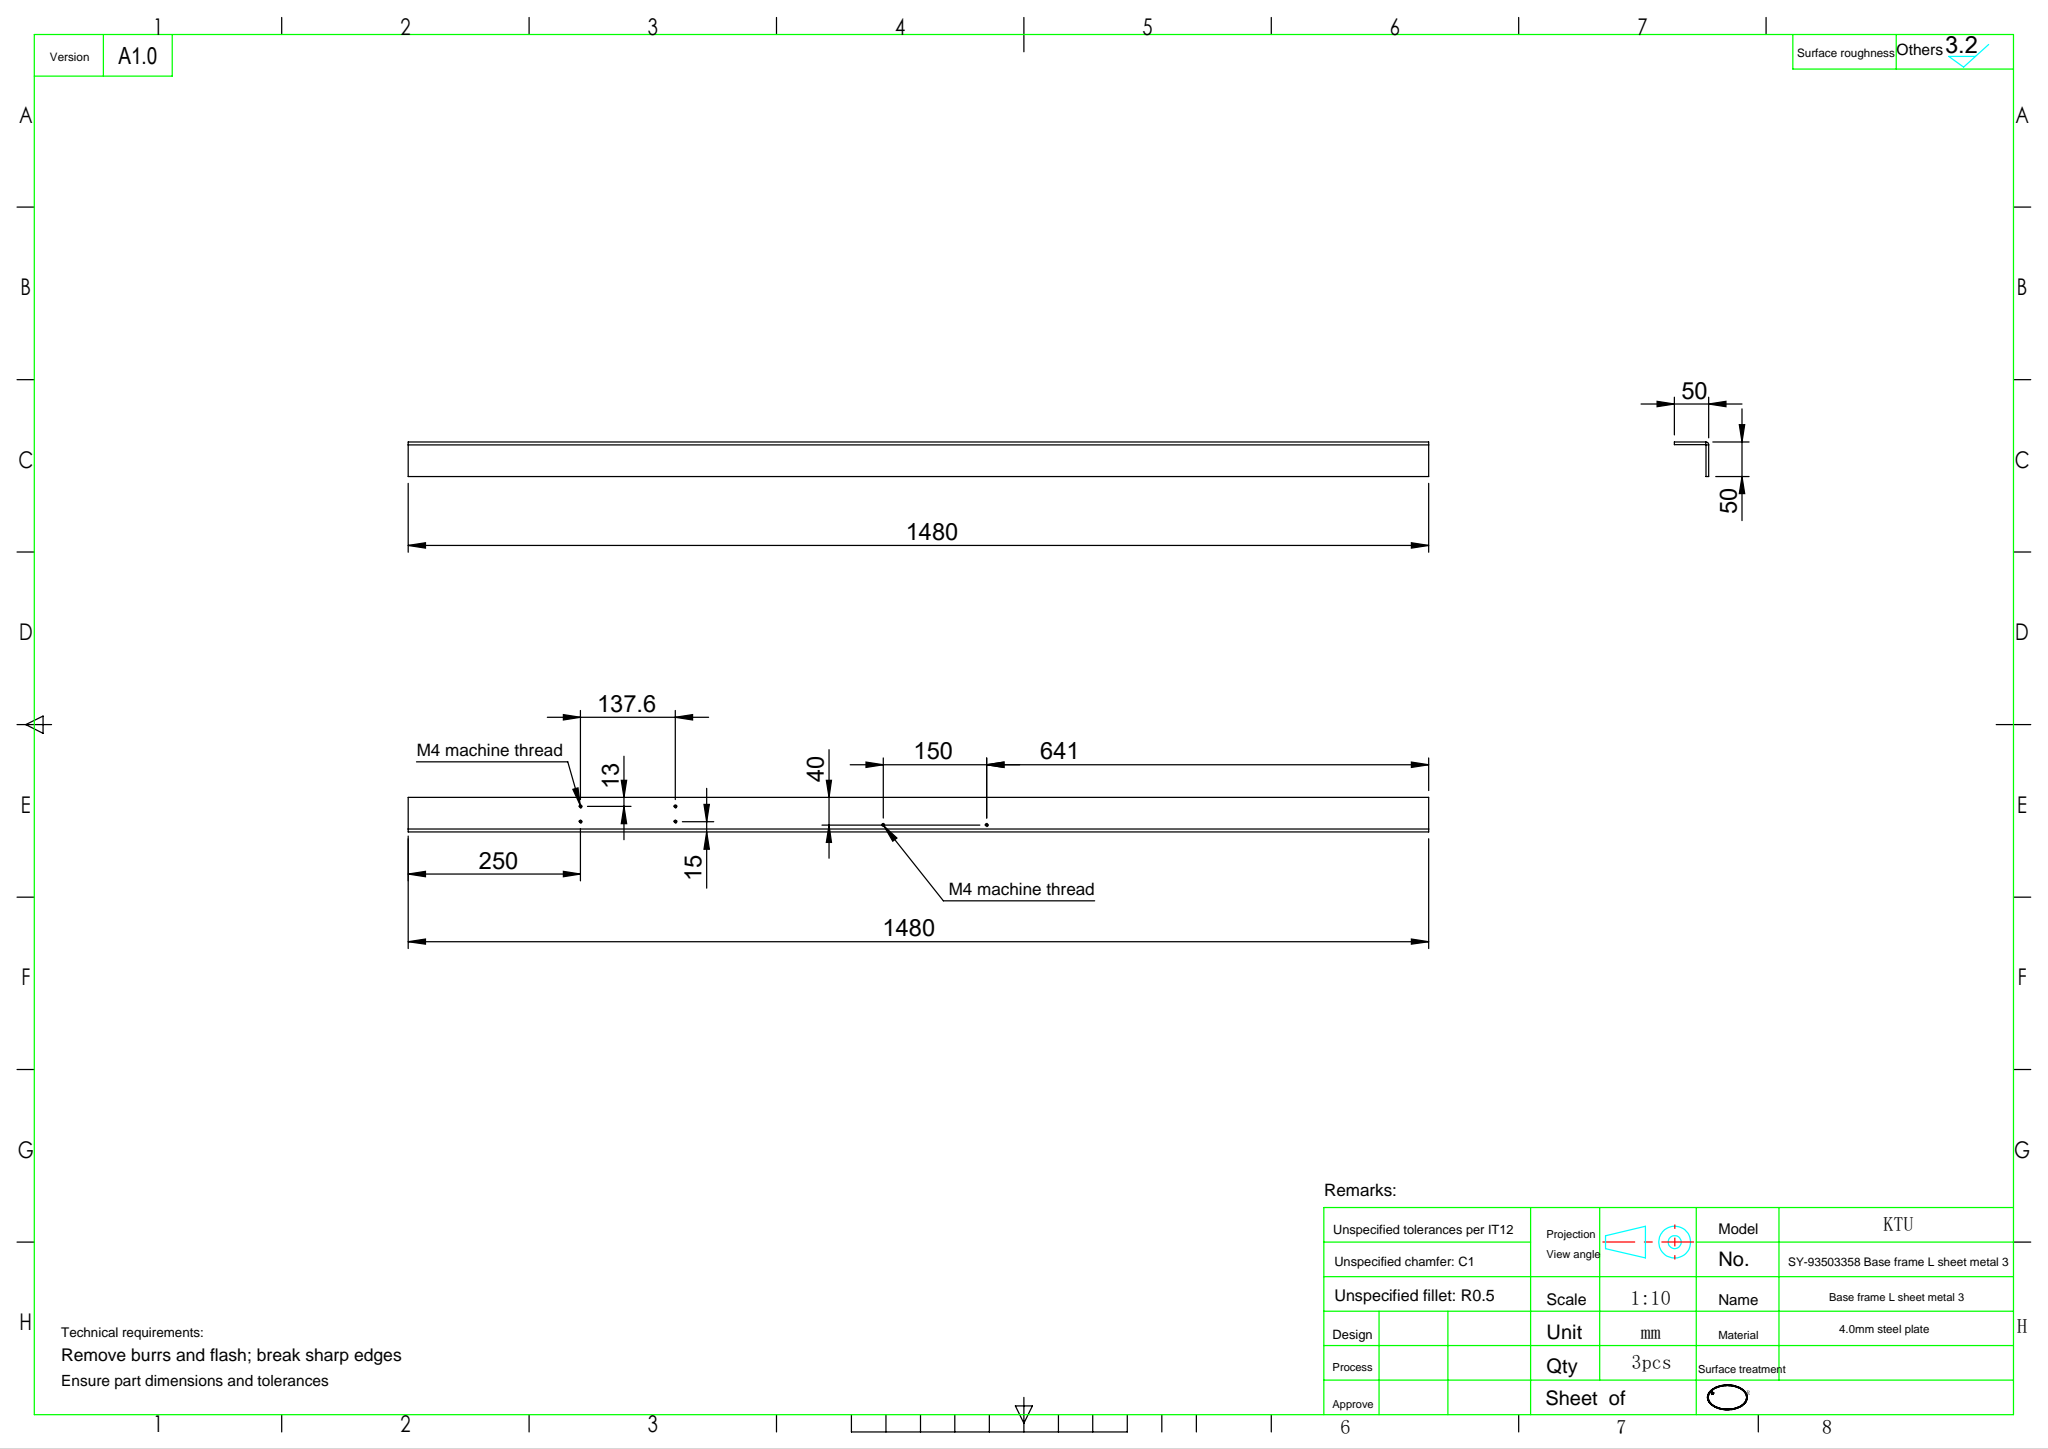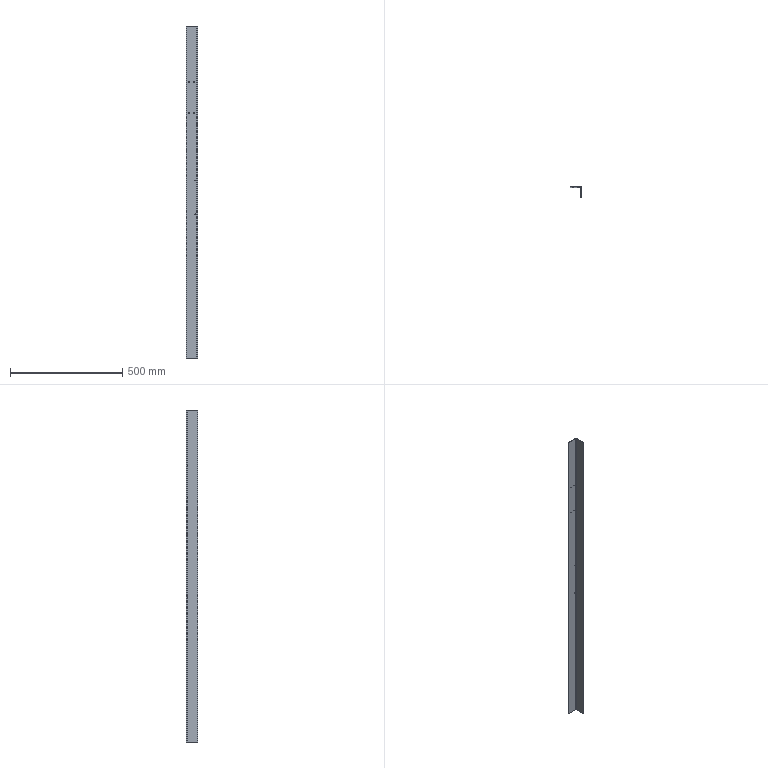Part | SolidWorks | features Cut 2, FlatPattern 1, SMBaseFlange 1, SheetMetal 1 | 1 solid | 26 faces | box 50 x 50 x 1480 mm | volume 562525 mm3 | cylinder 14 | plane 12 | commonest cylinder face diameters 3.3 x8 3.299 x4 0.4 x1 8.4 x1
STEP:
#1=CARTESIAN_POINT('',(-15.,-4.,1228.351));
#2=VERTEX_POINT('',#1);
#3=CARTESIAN_POINT('',(-15.,-4.,1231.649));
#4=VERTEX_POINT('',#3);
#5=CARTESIAN_POINT('',(-15.,-4.,1230.));
#6=DIRECTION('',(0.,1.,0.));
#7=DIRECTION('',(0.,0.,1.));
#8=AXIS2_PLACEMENT_3D('',#5,#6,#7);
#9=CIRCLE('',#8,1.649);
#10=EDGE_CURVE('',#2,#4,#9,.T.);
#11=ORIENTED_EDGE('',*,*,#10,.F.);
#12=CARTESIAN_POINT('',(-15.,0.,1228.351));
#13=VERTEX_POINT('',#12);
#14=CARTESIAN_POINT('',(-15.,-10.,1228.351));
#15=DIRECTION('',(0.,1.,0.));
#16=VECTOR('',#15,1000.);
#17=LINE('',#14,#16);
#18=EDGE_CURVE('',#2,#13,#17,.T.);
#19=ORIENTED_EDGE('',*,*,#18,.T.);
#20=CARTESIAN_POINT('',(-15.,0.,1231.649));
#21=VERTEX_POINT('',#20);
#22=CARTESIAN_POINT('',(-15.,0.,1230.));
#23=DIRECTION('',(0.,1.,0.));
#24=DIRECTION('',(0.,0.,1.));
#25=AXIS2_PLACEMENT_3D('',#22,#23,#24);
#26=CIRCLE('',#25,1.649);
#27=EDGE_CURVE('',#13,#21,#26,.T.);
#28=ORIENTED_EDGE('',*,*,#27,.T.);
#29=CARTESIAN_POINT('',(-15.,-10.,1231.649));
#30=DIRECTION('',(0.,1.,0.));
#31=VECTOR('',#30,1000.);
#32=LINE('',#29,#31);
#33=EDGE_CURVE('',#4,#21,#32,.T.);
#34=ORIENTED_EDGE('',*,*,#33,.F.);
#35=EDGE_LOOP('',(#11,#19,#28,#34));
#36=FACE_OUTER_BOUND('',#35,.T.);
#37=CARTESIAN_POINT('',(-15.,-10.,1230.));
#38=DIRECTION('',(0.,1.,0.));
#39=DIRECTION('',(0.,0.,1.));
#40=AXIS2_PLACEMENT_3D('',#37,#38,#39);
#41=CYLINDRICAL_SURFACE('',#40,1.649);
#42=ADVANCED_FACE('',(#36),#41,.F.);
#43=CARTESIAN_POINT('',(-15.,-4.,1090.751));
#44=VERTEX_POINT('',#43);
#45=CARTESIAN_POINT('',(-15.,-4.,1094.049));
#46=VERTEX_POINT('',#45);
#47=CARTESIAN_POINT('',(-15.,-4.,1092.4));
#48=DIRECTION('',(0.,1.,0.));
#49=DIRECTION('',(0.,0.,1.));
#50=AXIS2_PLACEMENT_3D('',#47,#48,#49);
#51=CIRCLE('',#50,1.649);
#52=EDGE_CURVE('',#44,#46,#51,.T.);
#53=ORIENTED_EDGE('',*,*,#52,.F.);
#54=CARTESIAN_POINT('',(-15.,0.,1090.751));
#55=VERTEX_POINT('',#54);
#56=CARTESIAN_POINT('',(-15.,-10.,1090.751));
#57=DIRECTION('',(0.,1.,0.));
#58=VECTOR('',#57,1000.);
#59=LINE('',#56,#58);
#60=EDGE_CURVE('',#44,#55,#59,.T.);
#61=ORIENTED_EDGE('',*,*,#60,.T.);
#62=CARTESIAN_POINT('',(-15.,0.,1094.049));
#63=VERTEX_POINT('',#62);
#64=CARTESIAN_POINT('',(-15.,0.,1092.4));
#65=DIRECTION('',(0.,1.,0.));
#66=DIRECTION('',(0.,0.,1.));
#67=AXIS2_PLACEMENT_3D('',#64,#65,#66);
#68=CIRCLE('',#67,1.649);
#69=EDGE_CURVE('',#55,#63,#68,.T.);
#70=ORIENTED_EDGE('',*,*,#69,.T.);
#71=CARTESIAN_POINT('',(-15.,-10.,1094.049));
#72=DIRECTION('',(0.,1.,0.));
#73=VECTOR('',#72,1000.);
#74=LINE('',#71,#73);
#75=EDGE_CURVE('',#46,#63,#74,.T.);
#76=ORIENTED_EDGE('',*,*,#75,.F.);
#77=EDGE_LOOP('',(#53,#61,#70,#76));
#78=FACE_OUTER_BOUND('',#77,.T.);
#79=CARTESIAN_POINT('',(-15.,-10.,1092.4));
#80=DIRECTION('',(0.,1.,0.));
#81=DIRECTION('',(0.,0.,1.));
#82=AXIS2_PLACEMENT_3D('',#79,#80,#81);
#83=CYLINDRICAL_SURFACE('',#82,1.649);
#84=ADVANCED_FACE('',(#78),#83,.F.);
#85=CARTESIAN_POINT('',(-10.,-4.,639.35));
#86=VERTEX_POINT('',#85);
#87=CARTESIAN_POINT('',(-10.,-4.,642.65));
#88=VERTEX_POINT('',#87);
#89=CARTESIAN_POINT('',(-10.,-4.,641.));
#90=DIRECTION('',(0.,1.,0.));
#91=DIRECTION('',(0.,0.,1.));
#92=AXIS2_PLACEMENT_3D('',#89,#90,#91);
#93=CIRCLE('',#92,1.65);
#94=EDGE_CURVE('',#86,#88,#93,.T.);
#95=ORIENTED_EDGE('',*,*,#94,.F.);
#96=CARTESIAN_POINT('',(-10.,0.,639.35));
#97=VERTEX_POINT('',#96);
#98=CARTESIAN_POINT('',(-10.,-10.,639.35));
#99=DIRECTION('',(0.,1.,0.));
#100=VECTOR('',#99,1000.);
#101=LINE('',#98,#100);
#102=EDGE_CURVE('',#86,#97,#101,.T.);
#103=ORIENTED_EDGE('',*,*,#102,.T.);
#104=CARTESIAN_POINT('',(-10.,0.,642.65));
#105=VERTEX_POINT('',#104);
#106=CARTESIAN_POINT('',(-10.,0.,641.));
#107=DIRECTION('',(0.,1.,0.));
#108=DIRECTION('',(0.,0.,1.));
#109=AXIS2_PLACEMENT_3D('',#106,#107,#108);
#110=CIRCLE('',#109,1.65);
#111=EDGE_CURVE('',#97,#105,#110,.T.);
#112=ORIENTED_EDGE('',*,*,#111,.T.);
#113=CARTESIAN_POINT('',(-10.,-10.,642.65));
#114=DIRECTION('',(0.,1.,0.));
#115=VECTOR('',#114,1000.);
#116=LINE('',#113,#115);
#117=EDGE_CURVE('',#88,#105,#116,.T.);
#118=ORIENTED_EDGE('',*,*,#117,.F.);
#119=EDGE_LOOP('',(#95,#103,#112,#118));
#120=FACE_OUTER_BOUND('',#119,.T.);
#121=CARTESIAN_POINT('',(-10.,-10.,641.));
#122=DIRECTION('',(0.,1.,0.));
#123=DIRECTION('',(0.,0.,1.));
#124=AXIS2_PLACEMENT_3D('',#121,#122,#123);
#125=CYLINDRICAL_SURFACE('',#124,1.65);
#126=ADVANCED_FACE('',(#120),#125,.F.);
#127=CARTESIAN_POINT('',(-37.,-4.,1228.35));
#128=VERTEX_POINT('',#127);
#129=CARTESIAN_POINT('',(-37.,-4.,1231.65));
#130=VERTEX_POINT('',#129);
#131=CARTESIAN_POINT('',(-37.,-4.,1230.));
#132=DIRECTION('',(0.,1.,0.));
#133=DIRECTION('',(0.,0.,1.));
#134=AXIS2_PLACEMENT_3D('',#131,#132,#133);
#135=CIRCLE('',#134,1.65);
#136=EDGE_CURVE('',#128,#130,#135,.T.);
#137=ORIENTED_EDGE('',*,*,#136,.F.);
#138=CARTESIAN_POINT('',(-37.,0.,1228.35));
#139=VERTEX_POINT('',#138);
#140=CARTESIAN_POINT('',(-37.,-10.,1228.35));
#141=DIRECTION('',(0.,1.,0.));
#142=VECTOR('',#141,1000.);
#143=LINE('',#140,#142);
#144=EDGE_CURVE('',#128,#139,#143,.T.);
#145=ORIENTED_EDGE('',*,*,#144,.T.);
#146=CARTESIAN_POINT('',(-37.,0.,1231.65));
#147=VERTEX_POINT('',#146);
#148=CARTESIAN_POINT('',(-37.,0.,1230.));
#149=DIRECTION('',(0.,1.,0.));
#150=DIRECTION('',(0.,0.,1.));
#151=AXIS2_PLACEMENT_3D('',#148,#149,#150);
#152=CIRCLE('',#151,1.65);
#153=EDGE_CURVE('',#139,#147,#152,.T.);
#154=ORIENTED_EDGE('',*,*,#153,.T.);
#155=CARTESIAN_POINT('',(-37.,-10.,1231.65));
#156=DIRECTION('',(0.,1.,0.));
#157=VECTOR('',#156,1000.);
#158=LINE('',#155,#157);
#159=EDGE_CURVE('',#130,#147,#158,.T.);
#160=ORIENTED_EDGE('',*,*,#159,.F.);
#161=EDGE_LOOP('',(#137,#145,#154,#160));
#162=FACE_OUTER_BOUND('',#161,.T.);
#163=CARTESIAN_POINT('',(-37.,-10.,1230.));
#164=DIRECTION('',(0.,1.,0.));
#165=DIRECTION('',(0.,0.,1.));
#166=AXIS2_PLACEMENT_3D('',#163,#164,#165);
#167=CYLINDRICAL_SURFACE('',#166,1.65);
#168=ADVANCED_FACE('',(#162),#167,.F.);
#169=CARTESIAN_POINT('',(-37.,-4.,1090.75));
#170=VERTEX_POINT('',#169);
#171=CARTESIAN_POINT('',(-37.,-4.,1094.05));
#172=VERTEX_POINT('',#171);
#173=CARTESIAN_POINT('',(-37.,-4.,1092.4));
#174=DIRECTION('',(0.,1.,0.));
#175=DIRECTION('',(0.,0.,1.));
#176=AXIS2_PLACEMENT_3D('',#173,#174,#175);
#177=CIRCLE('',#176,1.65);
#178=EDGE_CURVE('',#170,#172,#177,.T.);
#179=ORIENTED_EDGE('',*,*,#178,.F.);
#180=CARTESIAN_POINT('',(-37.,0.,1090.75));
#181=VERTEX_POINT('',#180);
#182=CARTESIAN_POINT('',(-37.,-10.,1090.75));
#183=DIRECTION('',(0.,1.,0.));
#184=VECTOR('',#183,1000.);
#185=LINE('',#182,#184);
#186=EDGE_CURVE('',#170,#181,#185,.T.);
#187=ORIENTED_EDGE('',*,*,#186,.T.);
#188=CARTESIAN_POINT('',(-37.,0.,1094.05));
#189=VERTEX_POINT('',#188);
#190=CARTESIAN_POINT('',(-37.,0.,1092.4));
#191=DIRECTION('',(0.,1.,0.));
#192=DIRECTION('',(0.,0.,1.));
#193=AXIS2_PLACEMENT_3D('',#190,#191,#192);
#194=CIRCLE('',#193,1.65);
#195=EDGE_CURVE('',#181,#189,#194,.T.);
#196=ORIENTED_EDGE('',*,*,#195,.T.);
#197=CARTESIAN_POINT('',(-37.,-10.,1094.05));
#198=DIRECTION('',(0.,1.,0.));
#199=VECTOR('',#198,1000.);
#200=LINE('',#197,#199);
#201=EDGE_CURVE('',#172,#189,#200,.T.);
#202=ORIENTED_EDGE('',*,*,#201,.F.);
#203=EDGE_LOOP('',(#179,#187,#196,#202));
#204=FACE_OUTER_BOUND('',#203,.T.);
#205=CARTESIAN_POINT('',(-37.,-10.,1092.4));
#206=DIRECTION('',(0.,1.,0.));
#207=DIRECTION('',(0.,0.,1.));
#208=AXIS2_PLACEMENT_3D('',#205,#206,#207);
#209=CYLINDRICAL_SURFACE('',#208,1.65);
#210=ADVANCED_FACE('',(#204),#209,.F.);
#211=CARTESIAN_POINT('',(-10.,-4.,789.35));
#212=VERTEX_POINT('',#211);
#213=CARTESIAN_POINT('',(-10.,-4.,792.65));
#214=VERTEX_POINT('',#213);
#215=CARTESIAN_POINT('',(-10.,-4.,791.));
#216=DIRECTION('',(0.,1.,0.));
#217=DIRECTION('',(0.,0.,1.));
#218=AXIS2_PLACEMENT_3D('',#215,#216,#217);
#219=CIRCLE('',#218,1.65);
#220=EDGE_CURVE('',#212,#214,#219,.T.);
#221=ORIENTED_EDGE('',*,*,#220,.F.);
#222=CARTESIAN_POINT('',(-10.,0.,789.35));
#223=VERTEX_POINT('',#222);
#224=CARTESIAN_POINT('',(-10.,-10.,789.35));
#225=DIRECTION('',(0.,1.,0.));
#226=VECTOR('',#225,1000.);
#227=LINE('',#224,#226);
#228=EDGE_CURVE('',#212,#223,#227,.T.);
#229=ORIENTED_EDGE('',*,*,#228,.T.);
#230=CARTESIAN_POINT('',(-10.,0.,792.65));
#231=VERTEX_POINT('',#230);
#232=CARTESIAN_POINT('',(-10.,0.,791.));
#233=DIRECTION('',(0.,1.,0.));
#234=DIRECTION('',(0.,0.,1.));
#235=AXIS2_PLACEMENT_3D('',#232,#233,#234);
#236=CIRCLE('',#235,1.65);
#237=EDGE_CURVE('',#223,#231,#236,.T.);
#238=ORIENTED_EDGE('',*,*,#237,.T.);
#239=CARTESIAN_POINT('',(-10.,-10.,792.65));
#240=DIRECTION('',(0.,1.,0.));
#241=VECTOR('',#240,1000.);
#242=LINE('',#239,#241);
#243=EDGE_CURVE('',#214,#231,#242,.T.);
#244=ORIENTED_EDGE('',*,*,#243,.F.);
#245=EDGE_LOOP('',(#221,#229,#238,#244));
#246=FACE_OUTER_BOUND('',#245,.T.);
#247=CARTESIAN_POINT('',(-10.,-10.,791.));
#248=DIRECTION('',(0.,1.,0.));
#249=DIRECTION('',(0.,0.,1.));
#250=AXIS2_PLACEMENT_3D('',#247,#248,#249);
#251=CYLINDRICAL_SURFACE('',#250,1.65);
#252=ADVANCED_FACE('',(#246),#251,.F.);
#253=CARTESIAN_POINT('',(0.,-4.2,1480.));
#254=VERTEX_POINT('',#253);
#255=CARTESIAN_POINT('',(-4.,-4.2,1480.));
#256=VERTEX_POINT('',#255);
#257=CARTESIAN_POINT('',(0.,-4.2,1480.));
#258=DIRECTION('',(-1.,0.,0.));
#259=VECTOR('',#258,1000.);
#260=LINE('',#257,#259);
#261=EDGE_CURVE('',#254,#256,#260,.T.);
#262=ORIENTED_EDGE('',*,*,#261,.F.);
#263=CARTESIAN_POINT('',(-4.2,0.,1480.));
#264=VERTEX_POINT('',#263);
#265=CARTESIAN_POINT('',(-4.2,-4.2,1480.));
#266=DIRECTION('',(0.,0.,-1.));
#267=DIRECTION('',(1.,0.,0.));
#268=AXIS2_PLACEMENT_3D('',#265,#266,#267);
#269=CIRCLE('',#268,4.2);
#270=EDGE_CURVE('',#264,#254,#269,.T.);
#271=ORIENTED_EDGE('',*,*,#270,.F.);
#272=CARTESIAN_POINT('',(-4.2,-4.,1480.));
#273=VERTEX_POINT('',#272);
#274=CARTESIAN_POINT('',(-4.2,-4.,1480.));
#275=DIRECTION('',(0.,1.,0.));
#276=VECTOR('',#275,1000.);
#277=LINE('',#274,#276);
#278=EDGE_CURVE('',#273,#264,#277,.T.);
#279=ORIENTED_EDGE('',*,*,#278,.F.);
#280=CARTESIAN_POINT('',(-4.2,-4.2,1480.));
#281=DIRECTION('',(0.,0.,-1.));
#282=DIRECTION('',(1.,0.,0.));
#283=AXIS2_PLACEMENT_3D('',#280,#281,#282);
#284=CIRCLE('',#283,0.2);
#285=EDGE_CURVE('',#273,#256,#284,.T.);
#286=ORIENTED_EDGE('',*,*,#285,.T.);
#287=EDGE_LOOP('',(#262,#271,#279,#286));
#288=FACE_OUTER_BOUND('',#287,.T.);
#289=CARTESIAN_POINT('',(0.,-4.2,1480.));
#290=DIRECTION('',(0.,0.,1.));
#291=DIRECTION('',(1.,0.,0.));
#292=AXIS2_PLACEMENT_3D('',#289,#290,#291);
#293=PLANE('',#292);
#294=ADVANCED_FACE('',(#288),#293,.T.);
#295=CARTESIAN_POINT('',(0.,-50.,1480.));
#296=VERTEX_POINT('',#295);
#297=CARTESIAN_POINT('',(0.,0.,1480.));
#298=DIRECTION('',(0.,-1.,0.));
#299=VECTOR('',#298,1000.);
#300=LINE('',#297,#299);
#301=EDGE_CURVE('',#254,#296,#300,.T.);
#302=ORIENTED_EDGE('',*,*,#301,.F.);
#303=ORIENTED_EDGE('',*,*,#261,.T.);
#304=CARTESIAN_POINT('',(-4.,-50.,1480.));
#305=VERTEX_POINT('',#304);
#306=CARTESIAN_POINT('',(-4.,0.,1480.));
#307=DIRECTION('',(0.,-1.,0.));
#308=VECTOR('',#307,1000.);
#309=LINE('',#306,#308);
#310=EDGE_CURVE('',#256,#305,#309,.T.);
#311=ORIENTED_EDGE('',*,*,#310,.T.);
#312=CARTESIAN_POINT('',(0.,-50.,1480.));
#313=DIRECTION('',(-1.,0.,0.));
#314=VECTOR('',#313,1000.);
#315=LINE('',#312,#314);
#316=EDGE_CURVE('',#296,#305,#315,.T.);
#317=ORIENTED_EDGE('',*,*,#316,.F.);
#318=EDGE_LOOP('',(#302,#303,#311,#317));
#319=FACE_OUTER_BOUND('',#318,.T.);
#320=CARTESIAN_POINT('',(-4.2,-4.,1480.));
#321=DIRECTION('',(0.,0.,1.));
#322=DIRECTION('',(1.,0.,0.));
#323=AXIS2_PLACEMENT_3D('',#320,#321,#322);
#324=PLANE('',#323);
#325=ADVANCED_FACE('',(#319),#324,.T.);
#326=CARTESIAN_POINT('',(-4.2,0.,0.));
#327=VERTEX_POINT('',#326);
#328=CARTESIAN_POINT('',(-4.2,-4.,0.));
#329=VERTEX_POINT('',#328);
#330=CARTESIAN_POINT('',(-4.2,0.,0.));
#331=DIRECTION('',(0.,-1.,0.));
#332=VECTOR('',#331,1000.);
#333=LINE('',#330,#332);
#334=EDGE_CURVE('',#327,#329,#333,.T.);
#335=ORIENTED_EDGE('',*,*,#334,.F.);
#336=CARTESIAN_POINT('',(0.,-4.2,0.));
#337=VERTEX_POINT('',#336);
#338=CARTESIAN_POINT('',(-4.2,-4.2,0.));
#339=DIRECTION('',(0.,0.,-1.));
#340=DIRECTION('',(1.,0.,0.));
#341=AXIS2_PLACEMENT_3D('',#338,#339,#340);
#342=CIRCLE('',#341,4.2);
#343=EDGE_CURVE('',#327,#337,#342,.T.);
#344=ORIENTED_EDGE('',*,*,#343,.T.);
#345=CARTESIAN_POINT('',(-4.,-4.2,0.));
#346=VERTEX_POINT('',#345);
#347=CARTESIAN_POINT('',(-4.,-4.2,0.));
#348=DIRECTION('',(1.,0.,0.));
#349=VECTOR('',#348,1000.);
#350=LINE('',#347,#349);
#351=EDGE_CURVE('',#346,#337,#350,.T.);
#352=ORIENTED_EDGE('',*,*,#351,.F.);
#353=CARTESIAN_POINT('',(-4.2,-4.2,0.));
#354=DIRECTION('',(0.,0.,-1.));
#355=DIRECTION('',(1.,0.,0.));
#356=AXIS2_PLACEMENT_3D('',#353,#354,#355);
#357=CIRCLE('',#356,0.2);
#358=EDGE_CURVE('',#329,#346,#357,.T.);
#359=ORIENTED_EDGE('',*,*,#358,.F.);
#360=EDGE_LOOP('',(#335,#344,#352,#359));
#361=FACE_OUTER_BOUND('',#360,.T.);
#362=CARTESIAN_POINT('',(-4.2,0.,0.));
#363=DIRECTION('',(0.,0.,-1.));
#364=DIRECTION('',(-1.,0.,0.));
#365=AXIS2_PLACEMENT_3D('',#362,#363,#364);
#366=PLANE('',#365);
#367=ADVANCED_FACE('',(#361),#366,.T.);
#368=CARTESIAN_POINT('',(-50.,0.,0.));
#369=VERTEX_POINT('',#368);
#370=CARTESIAN_POINT('',(-50.,0.,0.));
#371=DIRECTION('',(1.,0.,0.));
#372=VECTOR('',#371,1000.);
#373=LINE('',#370,#372);
#374=EDGE_CURVE('',#369,#327,#373,.T.);
#375=ORIENTED_EDGE('',*,*,#374,.T.);
#376=ORIENTED_EDGE('',*,*,#334,.T.);
#377=CARTESIAN_POINT('',(-50.,-4.,0.));
#378=VERTEX_POINT('',#377);
#379=CARTESIAN_POINT('',(-50.,-4.,0.));
#380=DIRECTION('',(1.,0.,0.));
#381=VECTOR('',#380,1000.);
#382=LINE('',#379,#381);
#383=EDGE_CURVE('',#378,#329,#382,.T.);
#384=ORIENTED_EDGE('',*,*,#383,.F.);
#385=CARTESIAN_POINT('',(-50.,-4.,0.));
#386=DIRECTION('',(0.,1.,0.));
#387=VECTOR('',#386,1000.);
#388=LINE('',#385,#387);
#389=EDGE_CURVE('',#378,#369,#388,.T.);
#390=ORIENTED_EDGE('',*,*,#389,.T.);
#391=EDGE_LOOP('',(#375,#376,#384,#390));
#392=FACE_OUTER_BOUND('',#391,.T.);
#393=CARTESIAN_POINT('',(-4.,-4.2,0.));
#394=DIRECTION('',(0.,0.,-1.));
#395=DIRECTION('',(-1.,0.,0.));
#396=AXIS2_PLACEMENT_3D('',#393,#394,#395);
#397=PLANE('',#396);
#398=ADVANCED_FACE('',(#392),#397,.T.);
#399=CARTESIAN_POINT('',(-4.,-50.,0.));
#400=VERTEX_POINT('',#399);
#401=CARTESIAN_POINT('',(-4.,0.,0.));
#402=DIRECTION('',(0.,-1.,0.));
#403=VECTOR('',#402,1000.);
#404=LINE('',#401,#403);
#405=EDGE_CURVE('',#346,#400,#404,.T.);
#406=ORIENTED_EDGE('',*,*,#405,.T.);
#407=CARTESIAN_POINT('',(-4.,-50.,1480.));
#408=DIRECTION('',(0.,0.,-1.));
#409=VECTOR('',#408,1000.);
#410=LINE('',#407,#409);
#411=EDGE_CURVE('',#305,#400,#410,.T.);
#412=ORIENTED_EDGE('',*,*,#411,.F.);
#413=ORIENTED_EDGE('',*,*,#310,.F.);
#414=CARTESIAN_POINT('',(-4.,-4.2,1480.));
#415=DIRECTION('',(0.,0.,-1.));
#416=VECTOR('',#415,1000.);
#417=LINE('',#414,#416);
#418=EDGE_CURVE('',#256,#346,#417,.T.);
#419=ORIENTED_EDGE('',*,*,#418,.T.);
#420=EDGE_LOOP('',(#406,#412,#413,#419));
#421=FACE_OUTER_BOUND('',#420,.T.);
#422=CARTESIAN_POINT('',(-4.,0.,1480.));
#423=DIRECTION('',(1.,0.,0.));
#424=DIRECTION('',(0.,1.,0.));
#425=AXIS2_PLACEMENT_3D('',#422,#423,#424);
#426=PLANE('',#425);
#427=ADVANCED_FACE('',(#421),#426,.F.);
#428=CARTESIAN_POINT('',(0.,-50.,0.));
#429=VERTEX_POINT('',#428);
#430=CARTESIAN_POINT('',(0.,-50.,0.));
#431=DIRECTION('',(-1.,0.,0.));
#432=VECTOR('',#431,1000.);
#433=LINE('',#430,#432);
#434=EDGE_CURVE('',#429,#400,#433,.T.);
#435=ORIENTED_EDGE('',*,*,#434,.F.);
#436=CARTESIAN_POINT('',(0.,-50.,1480.));
#437=DIRECTION('',(0.,0.,-1.));
#438=VECTOR('',#437,1000.);
#439=LINE('',#436,#438);
#440=EDGE_CURVE('',#296,#429,#439,.T.);
#441=ORIENTED_EDGE('',*,*,#440,.F.);
#442=ORIENTED_EDGE('',*,*,#316,.T.);
#443=ORIENTED_EDGE('',*,*,#411,.T.);
#444=EDGE_LOOP('',(#435,#441,#442,#443));
#445=FACE_OUTER_BOUND('',#444,.T.);
#446=CARTESIAN_POINT('',(0.,-50.,1480.));
#447=DIRECTION('',(0.,-1.,0.));
#448=DIRECTION('',(0.,0.,-1.));
#449=AXIS2_PLACEMENT_3D('',#446,#447,#448);
#450=PLANE('',#449);
#451=ADVANCED_FACE('',(#445),#450,.T.);
#452=CARTESIAN_POINT('',(0.,0.,0.));
#453=DIRECTION('',(0.,-1.,0.));
#454=VECTOR('',#453,1000.);
#455=LINE('',#452,#454);
#456=EDGE_CURVE('',#337,#429,#455,.T.);
#457=ORIENTED_EDGE('',*,*,#456,.F.);
#458=CARTESIAN_POINT('',(0.,-4.2,1480.));
#459=DIRECTION('',(0.,0.,-1.));
#460=VECTOR('',#459,1000.);
#461=LINE('',#458,#460);
#462=EDGE_CURVE('',#254,#337,#461,.T.);
#463=ORIENTED_EDGE('',*,*,#462,.F.);
#464=ORIENTED_EDGE('',*,*,#301,.T.);
#465=ORIENTED_EDGE('',*,*,#440,.T.);
#466=EDGE_LOOP('',(#457,#463,#464,#465));
#467=FACE_OUTER_BOUND('',#466,.T.);
#468=CARTESIAN_POINT('',(0.,0.,1480.));
#469=DIRECTION('',(1.,0.,0.));
#470=DIRECTION('',(0.,1.,0.));
#471=AXIS2_PLACEMENT_3D('',#468,#469,#470);
#472=PLANE('',#471);
#473=ADVANCED_FACE('',(#467),#472,.T.);
#474=ORIENTED_EDGE('',*,*,#343,.F.);
#475=CARTESIAN_POINT('',(-4.2,0.,1480.));
#476=DIRECTION('',(0.,0.,-1.));
#477=VECTOR('',#476,1000.);
#478=LINE('',#475,#477);
#479=EDGE_CURVE('',#264,#327,#478,.T.);
#480=ORIENTED_EDGE('',*,*,#479,.F.);
#481=ORIENTED_EDGE('',*,*,#270,.T.);
#482=ORIENTED_EDGE('',*,*,#462,.T.);
#483=EDGE_LOOP('',(#474,#480,#481,#482));
#484=FACE_OUTER_BOUND('',#483,.T.);
#485=CARTESIAN_POINT('',(-4.2,-4.2,1480.));
#486=DIRECTION('',(0.,0.,-1.));
#487=DIRECTION('',(-1.,0.,0.));
#488=AXIS2_PLACEMENT_3D('',#485,#486,#487);
#489=CYLINDRICAL_SURFACE('',#488,4.2);
#490=ADVANCED_FACE('',(#484),#489,.T.);
#491=CARTESIAN_POINT('',(-15.,0.,1230.));
#492=DIRECTION('',(0.,1.,0.));
#493=DIRECTION('',(0.,0.,1.));
#494=AXIS2_PLACEMENT_3D('',#491,#492,#493);
#495=CIRCLE('',#494,1.649);
#496=EDGE_CURVE('',#21,#13,#495,.T.);
#497=ORIENTED_EDGE('',*,*,#496,.F.);
#498=ORIENTED_EDGE('',*,*,#27,.F.);
#499=EDGE_LOOP('',(#497,#498));
#500=FACE_BOUND('',#499,.T.);
#501=CARTESIAN_POINT('',(-15.,0.,1092.4));
#502=DIRECTION('',(0.,1.,0.));
#503=DIRECTION('',(0.,0.,1.));
#504=AXIS2_PLACEMENT_3D('',#501,#502,#503);
#505=CIRCLE('',#504,1.649);
#506=EDGE_CURVE('',#63,#55,#505,.T.);
#507=ORIENTED_EDGE('',*,*,#506,.F.);
#508=ORIENTED_EDGE('',*,*,#69,.F.);
#509=EDGE_LOOP('',(#507,#508));
#510=FACE_BOUND('',#509,.T.);
#511=CARTESIAN_POINT('',(-10.,0.,641.));
#512=DIRECTION('',(0.,1.,0.));
#513=DIRECTION('',(0.,0.,1.));
#514=AXIS2_PLACEMENT_3D('',#511,#512,#513);
#515=CIRCLE('',#514,1.65);
#516=EDGE_CURVE('',#105,#97,#515,.T.);
#517=ORIENTED_EDGE('',*,*,#516,.F.);
#518=ORIENTED_EDGE('',*,*,#111,.F.);
#519=EDGE_LOOP('',(#517,#518));
#520=FACE_BOUND('',#519,.T.);
#521=CARTESIAN_POINT('',(-37.,0.,1230.));
#522=DIRECTION('',(0.,1.,0.));
#523=DIRECTION('',(0.,0.,1.));
#524=AXIS2_PLACEMENT_3D('',#521,#522,#523);
#525=CIRCLE('',#524,1.65);
#526=EDGE_CURVE('',#147,#139,#525,.T.);
#527=ORIENTED_EDGE('',*,*,#526,.F.);
#528=ORIENTED_EDGE('',*,*,#153,.F.);
#529=EDGE_LOOP('',(#527,#528));
#530=FACE_BOUND('',#529,.T.);
#531=CARTESIAN_POINT('',(-37.,0.,1092.4));
#532=DIRECTION('',(0.,1.,0.));
#533=DIRECTION('',(0.,0.,1.));
#534=AXIS2_PLACEMENT_3D('',#531,#532,#533);
#535=CIRCLE('',#534,1.65);
#536=EDGE_CURVE('',#189,#181,#535,.T.);
#537=ORIENTED_EDGE('',*,*,#536,.F.);
#538=ORIENTED_EDGE('',*,*,#195,.F.);
#539=EDGE_LOOP('',(#537,#538));
#540=FACE_BOUND('',#539,.T.);
#541=CARTESIAN_POINT('',(-10.,0.,791.));
#542=DIRECTION('',(0.,1.,0.));
#543=DIRECTION('',(0.,0.,1.));
#544=AXIS2_PLACEMENT_3D('',#541,#542,#543);
#545=CIRCLE('',#544,1.65);
#546=EDGE_CURVE('',#231,#223,#545,.T.);
#547=ORIENTED_EDGE('',*,*,#546,.F.);
#548=ORIENTED_EDGE('',*,*,#237,.F.);
#549=EDGE_LOOP('',(#547,#548));
#550=FACE_BOUND('',#549,.T.);
#551=ORIENTED_EDGE('',*,*,#374,.F.);
#552=CARTESIAN_POINT('',(-50.,0.,1480.));
#553=VERTEX_POINT('',#552);
#554=CARTESIAN_POINT('',(-50.,0.,1480.));
#555=DIRECTION('',(0.,0.,-1.));
#556=VECTOR('',#555,1000.);
#557=LINE('',#554,#556);
#558=EDGE_CURVE('',#553,#369,#557,.T.);
#559=ORIENTED_EDGE('',*,*,#558,.F.);
#560=CARTESIAN_POINT('',(-50.,0.,1480.));
#561=DIRECTION('',(1.,0.,0.));
#562=VECTOR('',#561,1000.);
#563=LINE('',#560,#562);
#564=EDGE_CURVE('',#553,#264,#563,.T.);
#565=ORIENTED_EDGE('',*,*,#564,.T.);
#566=ORIENTED_EDGE('',*,*,#479,.T.);
#567=EDGE_LOOP('',(#551,#559,#565,#566));
#568=FACE_OUTER_BOUND('',#567,.T.);
#569=CARTESIAN_POINT('',(-50.,0.,1480.));
#570=DIRECTION('',(0.,1.,0.));
#571=DIRECTION('',(0.,0.,1.));
#572=AXIS2_PLACEMENT_3D('',#569,#570,#571);
#573=PLANE('',#572);
#574=ADVANCED_FACE('',(#500,#510,#520,#530,#540,#550,#568),#573,.T.);
#575=ORIENTED_EDGE('',*,*,#389,.F.);
#576=CARTESIAN_POINT('',(-50.,-4.,1480.));
#577=VERTEX_POINT('',#576);
#578=CARTESIAN_POINT('',(-50.,-4.,1480.));
#579=DIRECTION('',(0.,0.,-1.));
#580=VECTOR('',#579,1000.);
#581=LINE('',#578,#580);
#582=EDGE_CURVE('',#577,#378,#581,.T.);
#583=ORIENTED_EDGE('',*,*,#582,.F.);
#584=CARTESIAN_POINT('',(-50.,-4.,1480.));
#585=DIRECTION('',(0.,1.,0.));
#586=VECTOR('',#585,1000.);
#587=LINE('',#584,#586);
#588=EDGE_CURVE('',#577,#553,#587,.T.);
#589=ORIENTED_EDGE('',*,*,#588,.T.);
#590=ORIENTED_EDGE('',*,*,#558,.T.);
#591=EDGE_LOOP('',(#575,#583,#589,#590));
#592=FACE_OUTER_BOUND('',#591,.T.);
#593=CARTESIAN_POINT('',(-50.,-4.,1480.));
#594=DIRECTION('',(-1.,0.,0.));
#595=DIRECTION('',(0.,0.,1.));
#596=AXIS2_PLACEMENT_3D('',#593,#594,#595);
#597=PLANE('',#596);
#598=ADVANCED_FACE('',(#592),#597,.T.);
#599=CARTESIAN_POINT('',(-15.,-4.,1230.));
#600=DIRECTION('',(0.,1.,0.));
#601=DIRECTION('',(0.,0.,1.));
#602=AXIS2_PLACEMENT_3D('',#599,#600,#601);
#603=CIRCLE('',#602,1.649);
#604=EDGE_CURVE('',#4,#2,#603,.T.);
#605=ORIENTED_EDGE('',*,*,#604,.T.);
#606=ORIENTED_EDGE('',*,*,#10,.T.);
#607=EDGE_LOOP('',(#605,#606));
#608=FACE_BOUND('',#607,.T.);
#609=CARTESIAN_POINT('',(-15.,-4.,1092.4));
#610=DIRECTION('',(0.,1.,0.));
#611=DIRECTION('',(0.,0.,1.));
#612=AXIS2_PLACEMENT_3D('',#609,#610,#611);
#613=CIRCLE('',#612,1.649);
#614=EDGE_CURVE('',#46,#44,#613,.T.);
#615=ORIENTED_EDGE('',*,*,#614,.T.);
#616=ORIENTED_EDGE('',*,*,#52,.T.);
#617=EDGE_LOOP('',(#615,#616));
#618=FACE_BOUND('',#617,.T.);
#619=CARTESIAN_POINT('',(-10.,-4.,641.));
#620=DIRECTION('',(0.,1.,0.));
#621=DIRECTION('',(0.,0.,1.));
#622=AXIS2_PLACEMENT_3D('',#619,#620,#621);
#623=CIRCLE('',#622,1.65);
#624=EDGE_CURVE('',#88,#86,#623,.T.);
#625=ORIENTED_EDGE('',*,*,#624,.T.);
#626=ORIENTED_EDGE('',*,*,#94,.T.);
#627=EDGE_LOOP('',(#625,#626));
#628=FACE_BOUND('',#627,.T.);
#629=CARTESIAN_POINT('',(-37.,-4.,1230.));
#630=DIRECTION('',(0.,1.,0.));
#631=DIRECTION('',(0.,0.,1.));
#632=AXIS2_PLACEMENT_3D('',#629,#630,#631);
#633=CIRCLE('',#632,1.65);
#634=EDGE_CURVE('',#130,#128,#633,.T.);
#635=ORIENTED_EDGE('',*,*,#634,.T.);
#636=ORIENTED_EDGE('',*,*,#136,.T.);
#637=EDGE_LOOP('',(#635,#636));
#638=FACE_BOUND('',#637,.T.);
#639=CARTESIAN_POINT('',(-37.,-4.,1092.4));
#640=DIRECTION('',(0.,1.,0.));
#641=DIRECTION('',(0.,0.,1.));
#642=AXIS2_PLACEMENT_3D('',#639,#640,#641);
#643=CIRCLE('',#642,1.65);
#644=EDGE_CURVE('',#172,#170,#643,.T.);
#645=ORIENTED_EDGE('',*,*,#644,.T.);
#646=ORIENTED_EDGE('',*,*,#178,.T.);
#647=EDGE_LOOP('',(#645,#646));
#648=FACE_BOUND('',#647,.T.);
#649=CARTESIAN_POINT('',(-10.,-4.,791.));
#650=DIRECTION('',(0.,1.,0.));
#651=DIRECTION('',(0.,0.,1.));
#652=AXIS2_PLACEMENT_3D('',#649,#650,#651);
#653=CIRCLE('',#652,1.65);
#654=EDGE_CURVE('',#214,#212,#653,.T.);
#655=ORIENTED_EDGE('',*,*,#654,.T.);
#656=ORIENTED_EDGE('',*,*,#220,.T.);
#657=EDGE_LOOP('',(#655,#656));
#658=FACE_BOUND('',#657,.T.);
#659=ORIENTED_EDGE('',*,*,#383,.T.);
#660=CARTESIAN_POINT('',(-4.2,-4.,1480.));
#661=DIRECTION('',(0.,0.,-1.));
#662=VECTOR('',#661,1000.);
#663=LINE('',#660,#662);
#664=EDGE_CURVE('',#273,#329,#663,.T.);
#665=ORIENTED_EDGE('',*,*,#664,.F.);
#666=CARTESIAN_POINT('',(-50.,-4.,1480.));
#667=DIRECTION('',(1.,0.,0.));
#668=VECTOR('',#667,1000.);
#669=LINE('',#666,#668);
#670=EDGE_CURVE('',#577,#273,#669,.T.);
#671=ORIENTED_EDGE('',*,*,#670,.F.);
#672=ORIENTED_EDGE('',*,*,#582,.T.);
#673=EDGE_LOOP('',(#659,#665,#671,#672));
#674=FACE_OUTER_BOUND('',#673,.T.);
#675=CARTESIAN_POINT('',(-50.,-4.,1480.));
#676=DIRECTION('',(0.,1.,0.));
#677=DIRECTION('',(0.,0.,1.));
#678=AXIS2_PLACEMENT_3D('',#675,#676,#677);
#679=PLANE('',#678);
#680=ADVANCED_FACE('',(#608,#618,#628,#638,#648,#658,#674),#679,.F.);
#681=ORIENTED_EDGE('',*,*,#358,.T.);
#682=ORIENTED_EDGE('',*,*,#418,.F.);
#683=ORIENTED_EDGE('',*,*,#285,.F.);
#684=ORIENTED_EDGE('',*,*,#664,.T.);
#685=EDGE_LOOP('',(#681,#682,#683,#684));
#686=FACE_OUTER_BOUND('',#685,.T.);
#687=CARTESIAN_POINT('',(-4.2,-4.2,1480.));
#688=DIRECTION('',(0.,0.,-1.));
#689=DIRECTION('',(-1.,0.,0.));
#690=AXIS2_PLACEMENT_3D('',#687,#688,#689);
#691=CYLINDRICAL_SURFACE('',#690,0.2);
#692=ADVANCED_FACE('',(#686),#691,.F.);
#693=ORIENTED_EDGE('',*,*,#670,.T.);
#694=ORIENTED_EDGE('',*,*,#278,.T.);
#695=ORIENTED_EDGE('',*,*,#564,.F.);
#696=ORIENTED_EDGE('',*,*,#588,.F.);
#697=EDGE_LOOP('',(#693,#694,#695,#696));
#698=FACE_OUTER_BOUND('',#697,.T.);
#699=CARTESIAN_POINT('',(-4.2,-4.2,1480.));
#700=DIRECTION('',(0.,0.,1.));
#701=DIRECTION('',(1.,0.,0.));
#702=AXIS2_PLACEMENT_3D('',#699,#700,#701);
#703=PLANE('',#702);
#704=ADVANCED_FACE('',(#698),#703,.T.);
#705=ORIENTED_EDGE('',*,*,#405,.F.);
#706=ORIENTED_EDGE('',*,*,#351,.T.);
#707=ORIENTED_EDGE('',*,*,#456,.T.);
#708=ORIENTED_EDGE('',*,*,#434,.T.);
#709=EDGE_LOOP('',(#705,#706,#707,#708));
#710=FACE_OUTER_BOUND('',#709,.T.);
#711=CARTESIAN_POINT('',(-4.2,-4.2,0.));
#712=DIRECTION('',(0.,0.,1.));
#713=DIRECTION('',(1.,0.,0.));
#714=AXIS2_PLACEMENT_3D('',#711,#712,#713);
#715=PLANE('',#714);
#716=ADVANCED_FACE('',(#710),#715,.F.);
#717=ORIENTED_EDGE('',*,*,#228,.F.);
#718=ORIENTED_EDGE('',*,*,#654,.F.);
#719=ORIENTED_EDGE('',*,*,#243,.T.);
#720=ORIENTED_EDGE('',*,*,#546,.T.);
#721=EDGE_LOOP('',(#717,#718,#719,#720));
#722=FACE_OUTER_BOUND('',#721,.T.);
#723=CARTESIAN_POINT('',(-10.,-10.,791.));
#724=DIRECTION('',(0.,1.,0.));
#725=DIRECTION('',(0.,0.,1.));
#726=AXIS2_PLACEMENT_3D('',#723,#724,#725);
#727=CYLINDRICAL_SURFACE('',#726,1.65);
#728=ADVANCED_FACE('',(#722),#727,.F.);
#729=ORIENTED_EDGE('',*,*,#186,.F.);
#730=ORIENTED_EDGE('',*,*,#644,.F.);
#731=ORIENTED_EDGE('',*,*,#201,.T.);
#732=ORIENTED_EDGE('',*,*,#536,.T.);
#733=EDGE_LOOP('',(#729,#730,#731,#732));
#734=FACE_OUTER_BOUND('',#733,.T.);
#735=CARTESIAN_POINT('',(-37.,-10.,1092.4));
#736=DIRECTION('',(0.,1.,0.));
#737=DIRECTION('',(0.,0.,1.));
#738=AXIS2_PLACEMENT_3D('',#735,#736,#737);
#739=CYLINDRICAL_SURFACE('',#738,1.65);
#740=ADVANCED_FACE('',(#734),#739,.F.);
#741=ORIENTED_EDGE('',*,*,#144,.F.);
#742=ORIENTED_EDGE('',*,*,#634,.F.);
#743=ORIENTED_EDGE('',*,*,#159,.T.);
#744=ORIENTED_EDGE('',*,*,#526,.T.);
#745=EDGE_LOOP('',(#741,#742,#743,#744));
#746=FACE_OUTER_BOUND('',#745,.T.);
#747=CARTESIAN_POINT('',(-37.,-10.,1230.));
#748=DIRECTION('',(0.,1.,0.));
#749=DIRECTION('',(0.,0.,1.));
#750=AXIS2_PLACEMENT_3D('',#747,#748,#749);
#751=CYLINDRICAL_SURFACE('',#750,1.65);
#752=ADVANCED_FACE('',(#746),#751,.F.);
#753=ORIENTED_EDGE('',*,*,#102,.F.);
#754=ORIENTED_EDGE('',*,*,#624,.F.);
#755=ORIENTED_EDGE('',*,*,#117,.T.);
#756=ORIENTED_EDGE('',*,*,#516,.T.);
#757=EDGE_LOOP('',(#753,#754,#755,#756));
#758=FACE_OUTER_BOUND('',#757,.T.);
#759=CARTESIAN_POINT('',(-10.,-10.,641.));
#760=DIRECTION('',(0.,1.,0.));
#761=DIRECTION('',(0.,0.,1.));
#762=AXIS2_PLACEMENT_3D('',#759,#760,#761);
#763=CYLINDRICAL_SURFACE('',#762,1.65);
#764=ADVANCED_FACE('',(#758),#763,.F.);
#765=ORIENTED_EDGE('',*,*,#60,.F.);
#766=ORIENTED_EDGE('',*,*,#614,.F.);
#767=ORIENTED_EDGE('',*,*,#75,.T.);
#768=ORIENTED_EDGE('',*,*,#506,.T.);
#769=EDGE_LOOP('',(#765,#766,#767,#768));
#770=FACE_OUTER_BOUND('',#769,.T.);
#771=CARTESIAN_POINT('',(-15.,-10.,1092.4));
#772=DIRECTION('',(0.,1.,0.));
#773=DIRECTION('',(0.,0.,1.));
#774=AXIS2_PLACEMENT_3D('',#771,#772,#773);
#775=CYLINDRICAL_SURFACE('',#774,1.649);
#776=ADVANCED_FACE('',(#770),#775,.F.);
#777=ORIENTED_EDGE('',*,*,#18,.F.);
#778=ORIENTED_EDGE('',*,*,#604,.F.);
#779=ORIENTED_EDGE('',*,*,#33,.T.);
#780=ORIENTED_EDGE('',*,*,#496,.T.);
#781=EDGE_LOOP('',(#777,#778,#779,#780));
#782=FACE_OUTER_BOUND('',#781,.T.);
#783=CARTESIAN_POINT('',(-15.,-10.,1230.));
#784=DIRECTION('',(0.,1.,0.));
#785=DIRECTION('',(0.,0.,1.));
#786=AXIS2_PLACEMENT_3D('',#783,#784,#785);
#787=CYLINDRICAL_SURFACE('',#786,1.649);
#788=ADVANCED_FACE('',(#782),#787,.F.);
#789=CLOSED_SHELL('',(#42,#84,#126,#168,#210,#252,#294,#325,#367,#398,#427,#451,#473,#490,#574,#598,#680,#692,#704,#716,#728,#740,#752,#764,#776,#788));
#790=MANIFOLD_SOLID_BREP('',#789);
#791=CARTESIAN_POINT('',(0.,0.,0.));
#792=DIRECTION('',(0.,0.,1.));
#793=DIRECTION('',(1.,0.,0.));
#794=AXIS2_PLACEMENT_3D('',#791,#792,#793);
#795=(LENGTH_UNIT()NAMED_UNIT(*)SI_UNIT(.MILLI.,.METRE.));
#796=UNCERTAINTY_MEASURE_WITH_UNIT(LENGTH_MEASURE(0.00001),#795,'','');
#797=(NAMED_UNIT(*)PLANE_ANGLE_UNIT()SI_UNIT($,.RADIAN.));
#798=(NAMED_UNIT(*)SI_UNIT($,.STERADIAN.)SOLID_ANGLE_UNIT());
#799=(GEOMETRIC_REPRESENTATION_CONTEXT(3)GLOBAL_UNCERTAINTY_ASSIGNED_CONTEXT((#796))GLOBAL_UNIT_ASSIGNED_CONTEXT((#795,#797,#798))REPRESENTATION_CONTEXT('',''));
#800=ADVANCED_BREP_SHAPE_REPRESENTATION('',(#790,#794),#799);